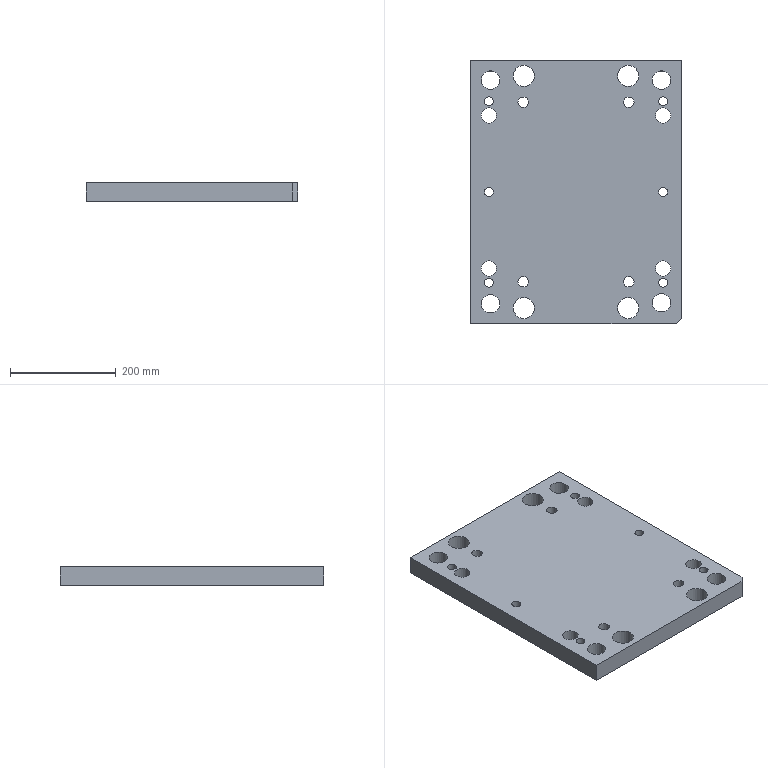Part | STEP file | SL2-MOLD_id734_xmt_txt | 1 solid | 29 faces | box 400 x 500 x 35 mm | volume 6503504 mm3 | cylinder 22 | plane 7 | commonest cylinder face diameters 17 x6 20 x4 29 x4 35 x4 40 x4
STEP:
#1=CARTESIAN_POINT('',(-200.,-160.,-114.));
#2=VERTEX_POINT('',#1);
#3=CARTESIAN_POINT('',(190.,-160.,-114.));
#4=VERTEX_POINT('',#3);
#5=CARTESIAN_POINT('',(0.,-160.,-114.));
#6=DIRECTION('',(1.,0.,0.));
#7=VECTOR('',#6,1.);
#8=LINE('',#5,#7);
#9=EDGE_CURVE('',#2,#4,#8,.T.);
#10=ORIENTED_EDGE('',*,*,#9,.T.);
#11=CARTESIAN_POINT('',(190.,-160.,-79.));
#12=VERTEX_POINT('',#11);
#13=CARTESIAN_POINT('',(190.,-160.,-114.));
#14=DIRECTION('',(0.,0.,1.));
#15=VECTOR('',#14,1.);
#16=LINE('',#13,#15);
#17=EDGE_CURVE('',#4,#12,#16,.T.);
#18=ORIENTED_EDGE('',*,*,#17,.T.);
#19=CARTESIAN_POINT('',(-200.,-160.,-79.));
#20=VERTEX_POINT('',#19);
#21=CARTESIAN_POINT('',(0.,-160.,-79.));
#22=DIRECTION('',(1.,0.,0.));
#23=VECTOR('',#22,1.);
#24=LINE('',#21,#23);
#25=EDGE_CURVE('',#20,#12,#24,.T.);
#26=ORIENTED_EDGE('',*,*,#25,.F.);
#27=CARTESIAN_POINT('',(-200.,-160.,-114.));
#28=DIRECTION('',(0.,0.,1.));
#29=VECTOR('',#28,1.);
#30=LINE('',#27,#29);
#31=EDGE_CURVE('',#2,#20,#30,.T.);
#32=ORIENTED_EDGE('',*,*,#31,.F.);
#33=EDGE_LOOP('',(#10,#18,#26,#32));
#34=FACE_OUTER_BOUND('',#33,.T.);
#35=CARTESIAN_POINT('',(0.,-160.,-114.));
#36=DIRECTION('',(0.,-1.,0.));
#37=DIRECTION('',(0.,0.,-1.));
#38=AXIS2_PLACEMENT_3D('',#35,#36,#37);
#39=PLANE('',#38);
#40=ADVANCED_FACE('',(#34),#39,.T.);
#41=CARTESIAN_POINT('',(-200.,340.,-79.));
#42=VERTEX_POINT('',#41);
#43=CARTESIAN_POINT('',(-200.,0.,-79.));
#44=DIRECTION('',(0.,-1.,0.));
#45=VECTOR('',#44,1.);
#46=LINE('',#43,#45);
#47=EDGE_CURVE('',#42,#20,#46,.T.);
#48=ORIENTED_EDGE('',*,*,#47,.F.);
#49=CARTESIAN_POINT('',(-200.,340.,-114.));
#50=VERTEX_POINT('',#49);
#51=CARTESIAN_POINT('',(-200.,340.,-114.));
#52=DIRECTION('',(0.,0.,1.));
#53=VECTOR('',#52,1.);
#54=LINE('',#51,#53);
#55=EDGE_CURVE('',#50,#42,#54,.T.);
#56=ORIENTED_EDGE('',*,*,#55,.F.);
#57=CARTESIAN_POINT('',(-200.,0.,-114.));
#58=DIRECTION('',(0.,-1.,0.));
#59=VECTOR('',#58,1.);
#60=LINE('',#57,#59);
#61=EDGE_CURVE('',#50,#2,#60,.T.);
#62=ORIENTED_EDGE('',*,*,#61,.T.);
#63=ORIENTED_EDGE('',*,*,#31,.T.);
#64=EDGE_LOOP('',(#48,#56,#62,#63));
#65=FACE_OUTER_BOUND('',#64,.T.);
#66=CARTESIAN_POINT('',(-200.,0.,-114.));
#67=DIRECTION('',(-1.,0.,0.));
#68=DIRECTION('',(0.,0.,1.));
#69=AXIS2_PLACEMENT_3D('',#66,#67,#68);
#70=PLANE('',#69);
#71=ADVANCED_FACE('',(#65),#70,.T.);
#72=CARTESIAN_POINT('',(200.,340.,-79.));
#73=VERTEX_POINT('',#72);
#74=CARTESIAN_POINT('',(0.,340.,-79.));
#75=DIRECTION('',(-1.,0.,0.));
#76=VECTOR('',#75,1.);
#77=LINE('',#74,#76);
#78=EDGE_CURVE('',#73,#42,#77,.T.);
#79=ORIENTED_EDGE('',*,*,#78,.F.);
#80=CARTESIAN_POINT('',(200.,340.,-114.));
#81=VERTEX_POINT('',#80);
#82=CARTESIAN_POINT('',(200.,340.,-114.));
#83=DIRECTION('',(0.,0.,1.));
#84=VECTOR('',#83,1.);
#85=LINE('',#82,#84);
#86=EDGE_CURVE('',#81,#73,#85,.T.);
#87=ORIENTED_EDGE('',*,*,#86,.F.);
#88=CARTESIAN_POINT('',(0.,340.,-114.));
#89=DIRECTION('',(-1.,0.,0.));
#90=VECTOR('',#89,1.);
#91=LINE('',#88,#90);
#92=EDGE_CURVE('',#81,#50,#91,.T.);
#93=ORIENTED_EDGE('',*,*,#92,.T.);
#94=ORIENTED_EDGE('',*,*,#55,.T.);
#95=EDGE_LOOP('',(#79,#87,#93,#94));
#96=FACE_OUTER_BOUND('',#95,.T.);
#97=CARTESIAN_POINT('',(0.,340.,-114.));
#98=DIRECTION('',(0.,1.,0.));
#99=DIRECTION('',(0.,0.,1.));
#100=AXIS2_PLACEMENT_3D('',#97,#98,#99);
#101=PLANE('',#100);
#102=ADVANCED_FACE('',(#96),#101,.T.);
#103=CARTESIAN_POINT('',(200.,-150.,-79.));
#104=VERTEX_POINT('',#103);
#105=CARTESIAN_POINT('',(200.,0.,-79.));
#106=DIRECTION('',(0.,1.,0.));
#107=VECTOR('',#106,1.);
#108=LINE('',#105,#107);
#109=EDGE_CURVE('',#104,#73,#108,.T.);
#110=ORIENTED_EDGE('',*,*,#109,.F.);
#111=CARTESIAN_POINT('',(200.,-150.,-114.));
#112=VERTEX_POINT('',#111);
#113=CARTESIAN_POINT('',(200.,-150.,-114.));
#114=DIRECTION('',(0.,0.,-1.));
#115=VECTOR('',#114,1.);
#116=LINE('',#113,#115);
#117=EDGE_CURVE('',#104,#112,#116,.T.);
#118=ORIENTED_EDGE('',*,*,#117,.T.);
#119=CARTESIAN_POINT('',(200.,0.,-114.));
#120=DIRECTION('',(0.,1.,0.));
#121=VECTOR('',#120,1.);
#122=LINE('',#119,#121);
#123=EDGE_CURVE('',#112,#81,#122,.T.);
#124=ORIENTED_EDGE('',*,*,#123,.T.);
#125=ORIENTED_EDGE('',*,*,#86,.T.);
#126=EDGE_LOOP('',(#110,#118,#124,#125));
#127=FACE_OUTER_BOUND('',#126,.T.);
#128=CARTESIAN_POINT('',(200.,0.,-114.));
#129=DIRECTION('',(1.,0.,0.));
#130=DIRECTION('',(0.,0.,-1.));
#131=AXIS2_PLACEMENT_3D('',#128,#129,#130);
#132=PLANE('',#131);
#133=ADVANCED_FACE('',(#127),#132,.T.);
#134=CARTESIAN_POINT('',(-90.,260.,-114.));
#135=VERTEX_POINT('',#134);
#136=CARTESIAN_POINT('',(-100.,260.,-114.));
#137=DIRECTION('',(0.,0.,-1.));
#138=DIRECTION('',(1.,0.,0.));
#139=AXIS2_PLACEMENT_3D('',#136,#137,#138);
#140=CIRCLE('',#139,10.);
#141=EDGE_CURVE('',#135,#135,#140,.T.);
#142=ORIENTED_EDGE('',*,*,#141,.F.);
#143=EDGE_LOOP('',(#142));
#144=FACE_BOUND('',#143,.T.);
#145=CARTESIAN_POINT('',(110.,-80.,-114.));
#146=VERTEX_POINT('',#145);
#147=CARTESIAN_POINT('',(100.,-80.,-114.));
#148=DIRECTION('',(0.,0.,-1.));
#149=DIRECTION('',(1.,0.,0.));
#150=AXIS2_PLACEMENT_3D('',#147,#148,#149);
#151=CIRCLE('',#150,10.);
#152=EDGE_CURVE('',#146,#146,#151,.T.);
#153=ORIENTED_EDGE('',*,*,#152,.F.);
#154=EDGE_LOOP('',(#153));
#155=FACE_BOUND('',#154,.T.);
#156=CARTESIAN_POINT('',(-90.,-80.,-114.));
#157=VERTEX_POINT('',#156);
#158=CARTESIAN_POINT('',(-100.,-80.,-114.));
#159=DIRECTION('',(0.,0.,-1.));
#160=DIRECTION('',(1.,0.,0.));
#161=AXIS2_PLACEMENT_3D('',#158,#159,#160);
#162=CIRCLE('',#161,10.);
#163=EDGE_CURVE('',#157,#157,#162,.T.);
#164=ORIENTED_EDGE('',*,*,#163,.F.);
#165=EDGE_LOOP('',(#164));
#166=FACE_BOUND('',#165,.T.);
#167=CARTESIAN_POINT('',(110.,260.,-114.));
#168=VERTEX_POINT('',#167);
#169=CARTESIAN_POINT('',(100.,260.,-114.));
#170=DIRECTION('',(0.,0.,-1.));
#171=DIRECTION('',(1.,0.,0.));
#172=AXIS2_PLACEMENT_3D('',#169,#170,#171);
#173=CIRCLE('',#172,10.);
#174=EDGE_CURVE('',#168,#168,#173,.T.);
#175=ORIENTED_EDGE('',*,*,#174,.F.);
#176=EDGE_LOOP('',(#175));
#177=FACE_BOUND('',#176,.T.);
#178=CARTESIAN_POINT('',(-79.,310.,-114.));
#179=VERTEX_POINT('',#178);
#180=CARTESIAN_POINT('',(-99.,310.,-114.));
#181=DIRECTION('',(0.,0.,-1.));
#182=DIRECTION('',(1.,0.,0.));
#183=AXIS2_PLACEMENT_3D('',#180,#181,#182);
#184=CIRCLE('',#183,20.);
#185=EDGE_CURVE('',#179,#179,#184,.T.);
#186=ORIENTED_EDGE('',*,*,#185,.F.);
#187=EDGE_LOOP('',(#186));
#188=FACE_BOUND('',#187,.T.);
#189=CARTESIAN_POINT('',(119.,310.,-114.));
#190=VERTEX_POINT('',#189);
#191=CARTESIAN_POINT('',(99.,310.,-114.));
#192=DIRECTION('',(0.,0.,-1.));
#193=DIRECTION('',(1.,0.,0.));
#194=AXIS2_PLACEMENT_3D('',#191,#192,#193);
#195=CIRCLE('',#194,20.);
#196=EDGE_CURVE('',#190,#190,#195,.T.);
#197=ORIENTED_EDGE('',*,*,#196,.F.);
#198=EDGE_LOOP('',(#197));
#199=FACE_BOUND('',#198,.T.);
#200=CARTESIAN_POINT('',(119.,-130.,-114.));
#201=VERTEX_POINT('',#200);
#202=CARTESIAN_POINT('',(99.,-130.,-114.));
#203=DIRECTION('',(0.,0.,-1.));
#204=DIRECTION('',(1.,0.,0.));
#205=AXIS2_PLACEMENT_3D('',#202,#203,#204);
#206=CIRCLE('',#205,20.);
#207=EDGE_CURVE('',#201,#201,#206,.T.);
#208=ORIENTED_EDGE('',*,*,#207,.F.);
#209=EDGE_LOOP('',(#208));
#210=FACE_BOUND('',#209,.T.);
#211=CARTESIAN_POINT('',(-79.,-130.,-114.));
#212=VERTEX_POINT('',#211);
#213=CARTESIAN_POINT('',(-99.,-130.,-114.));
#214=DIRECTION('',(0.,0.,-1.));
#215=DIRECTION('',(1.,0.,0.));
#216=AXIS2_PLACEMENT_3D('',#213,#214,#215);
#217=CIRCLE('',#216,20.);
#218=EDGE_CURVE('',#212,#212,#217,.T.);
#219=ORIENTED_EDGE('',*,*,#218,.F.);
#220=EDGE_LOOP('',(#219));
#221=FACE_BOUND('',#220,.T.);
#222=CARTESIAN_POINT('',(-156.5,-82.,-114.));
#223=VERTEX_POINT('',#222);
#224=CARTESIAN_POINT('',(-165.,-82.,-114.));
#225=DIRECTION('',(0.,0.,1.));
#226=DIRECTION('',(1.,0.,0.));
#227=AXIS2_PLACEMENT_3D('',#224,#225,#226);
#228=CIRCLE('',#227,8.5);
#229=EDGE_CURVE('',#223,#223,#228,.T.);
#230=ORIENTED_EDGE('',*,*,#229,.T.);
#231=EDGE_LOOP('',(#230));
#232=FACE_BOUND('',#231,.T.);
#233=CARTESIAN_POINT('',(-156.5,90.,-114.));
#234=VERTEX_POINT('',#233);
#235=CARTESIAN_POINT('',(-165.,90.,-114.));
#236=DIRECTION('',(0.,0.,1.));
#237=DIRECTION('',(1.,0.,0.));
#238=AXIS2_PLACEMENT_3D('',#235,#236,#237);
#239=CIRCLE('',#238,8.5);
#240=EDGE_CURVE('',#234,#234,#239,.T.);
#241=ORIENTED_EDGE('',*,*,#240,.T.);
#242=EDGE_LOOP('',(#241));
#243=FACE_BOUND('',#242,.T.);
#244=CARTESIAN_POINT('',(-156.5,262.,-114.));
#245=VERTEX_POINT('',#244);
#246=CARTESIAN_POINT('',(-165.,262.,-114.));
#247=DIRECTION('',(0.,0.,1.));
#248=DIRECTION('',(1.,0.,0.));
#249=AXIS2_PLACEMENT_3D('',#246,#247,#248);
#250=CIRCLE('',#249,8.5);
#251=EDGE_CURVE('',#245,#245,#250,.T.);
#252=ORIENTED_EDGE('',*,*,#251,.T.);
#253=EDGE_LOOP('',(#252));
#254=FACE_BOUND('',#253,.T.);
#255=CARTESIAN_POINT('',(173.5,262.,-114.));
#256=VERTEX_POINT('',#255);
#257=CARTESIAN_POINT('',(165.,262.,-114.));
#258=DIRECTION('',(0.,0.,1.));
#259=DIRECTION('',(1.,0.,0.));
#260=AXIS2_PLACEMENT_3D('',#257,#258,#259);
#261=CIRCLE('',#260,8.5);
#262=EDGE_CURVE('',#256,#256,#261,.T.);
#263=ORIENTED_EDGE('',*,*,#262,.T.);
#264=EDGE_LOOP('',(#263));
#265=FACE_BOUND('',#264,.T.);
#266=CARTESIAN_POINT('',(173.5,90.,-114.));
#267=VERTEX_POINT('',#266);
#268=CARTESIAN_POINT('',(165.,90.,-114.));
#269=DIRECTION('',(0.,0.,1.));
#270=DIRECTION('',(1.,0.,0.));
#271=AXIS2_PLACEMENT_3D('',#268,#269,#270);
#272=CIRCLE('',#271,8.5);
#273=EDGE_CURVE('',#267,#267,#272,.T.);
#274=ORIENTED_EDGE('',*,*,#273,.T.);
#275=EDGE_LOOP('',(#274));
#276=FACE_BOUND('',#275,.T.);
#277=CARTESIAN_POINT('',(173.5,-82.,-114.));
#278=VERTEX_POINT('',#277);
#279=CARTESIAN_POINT('',(165.,-82.,-114.));
#280=DIRECTION('',(0.,0.,1.));
#281=DIRECTION('',(1.,0.,0.));
#282=AXIS2_PLACEMENT_3D('',#279,#280,#281);
#283=CIRCLE('',#282,8.5);
#284=EDGE_CURVE('',#278,#278,#283,.T.);
#285=ORIENTED_EDGE('',*,*,#284,.T.);
#286=EDGE_LOOP('',(#285));
#287=FACE_BOUND('',#286,.T.);
#288=CARTESIAN_POINT('',(-150.5,-55.,-114.));
#289=VERTEX_POINT('',#288);
#290=CARTESIAN_POINT('',(-165.,-55.,-114.));
#291=DIRECTION('',(0.,0.,1.));
#292=DIRECTION('',(1.,0.,0.));
#293=AXIS2_PLACEMENT_3D('',#290,#291,#292);
#294=CIRCLE('',#293,14.5);
#295=EDGE_CURVE('',#289,#289,#294,.T.);
#296=ORIENTED_EDGE('',*,*,#295,.T.);
#297=EDGE_LOOP('',(#296));
#298=FACE_BOUND('',#297,.T.);
#299=CARTESIAN_POINT('',(179.5,-55.,-114.));
#300=VERTEX_POINT('',#299);
#301=CARTESIAN_POINT('',(165.,-55.,-114.));
#302=DIRECTION('',(0.,0.,1.));
#303=DIRECTION('',(1.,0.,0.));
#304=AXIS2_PLACEMENT_3D('',#301,#302,#303);
#305=CIRCLE('',#304,14.5);
#306=EDGE_CURVE('',#300,#300,#305,.T.);
#307=ORIENTED_EDGE('',*,*,#306,.T.);
#308=EDGE_LOOP('',(#307));
#309=FACE_BOUND('',#308,.T.);
#310=CARTESIAN_POINT('',(179.5,235.,-114.));
#311=VERTEX_POINT('',#310);
#312=CARTESIAN_POINT('',(165.,235.,-114.));
#313=DIRECTION('',(0.,0.,1.));
#314=DIRECTION('',(1.,0.,0.));
#315=AXIS2_PLACEMENT_3D('',#312,#313,#314);
#316=CIRCLE('',#315,14.5);
#317=EDGE_CURVE('',#311,#311,#316,.T.);
#318=ORIENTED_EDGE('',*,*,#317,.T.);
#319=EDGE_LOOP('',(#318));
#320=FACE_BOUND('',#319,.T.);
#321=CARTESIAN_POINT('',(-150.5,235.,-114.));
#322=VERTEX_POINT('',#321);
#323=CARTESIAN_POINT('',(-165.,235.,-114.));
#324=DIRECTION('',(0.,0.,1.));
#325=DIRECTION('',(1.,0.,0.));
#326=AXIS2_PLACEMENT_3D('',#323,#324,#325);
#327=CIRCLE('',#326,14.5);
#328=EDGE_CURVE('',#322,#322,#327,.T.);
#329=ORIENTED_EDGE('',*,*,#328,.T.);
#330=EDGE_LOOP('',(#329));
#331=FACE_BOUND('',#330,.T.);
#332=CARTESIAN_POINT('',(-144.5,-122.,-114.));
#333=VERTEX_POINT('',#332);
#334=CARTESIAN_POINT('',(-162.,-122.,-114.));
#335=DIRECTION('',(0.,0.,-1.));
#336=DIRECTION('',(1.,0.,0.));
#337=AXIS2_PLACEMENT_3D('',#334,#335,#336);
#338=CIRCLE('',#337,17.5);
#339=EDGE_CURVE('',#333,#333,#338,.T.);
#340=ORIENTED_EDGE('',*,*,#339,.F.);
#341=EDGE_LOOP('',(#340));
#342=FACE_BOUND('',#341,.T.);
#343=CARTESIAN_POINT('',(179.5,-120.,-114.));
#344=VERTEX_POINT('',#343);
#345=CARTESIAN_POINT('',(162.,-120.,-114.));
#346=DIRECTION('',(0.,0.,-1.));
#347=DIRECTION('',(1.,0.,0.));
#348=AXIS2_PLACEMENT_3D('',#345,#346,#347);
#349=CIRCLE('',#348,17.5);
#350=EDGE_CURVE('',#344,#344,#349,.T.);
#351=ORIENTED_EDGE('',*,*,#350,.F.);
#352=EDGE_LOOP('',(#351));
#353=FACE_BOUND('',#352,.T.);
#354=CARTESIAN_POINT('',(179.5,302.,-114.));
#355=VERTEX_POINT('',#354);
#356=CARTESIAN_POINT('',(162.,302.,-114.));
#357=DIRECTION('',(0.,0.,-1.));
#358=DIRECTION('',(1.,0.,0.));
#359=AXIS2_PLACEMENT_3D('',#356,#357,#358);
#360=CIRCLE('',#359,17.5);
#361=EDGE_CURVE('',#355,#355,#360,.T.);
#362=ORIENTED_EDGE('',*,*,#361,.F.);
#363=EDGE_LOOP('',(#362));
#364=FACE_BOUND('',#363,.T.);
#365=CARTESIAN_POINT('',(-144.5,302.,-114.));
#366=VERTEX_POINT('',#365);
#367=CARTESIAN_POINT('',(-162.,302.,-114.));
#368=DIRECTION('',(0.,0.,-1.));
#369=DIRECTION('',(1.,0.,0.));
#370=AXIS2_PLACEMENT_3D('',#367,#368,#369);
#371=CIRCLE('',#370,17.5);
#372=EDGE_CURVE('',#366,#366,#371,.T.);
#373=ORIENTED_EDGE('',*,*,#372,.F.);
#374=EDGE_LOOP('',(#373));
#375=FACE_BOUND('',#374,.T.);
#376=ORIENTED_EDGE('',*,*,#123,.F.);
#377=CARTESIAN_POINT('',(190.,-160.,-114.));
#378=DIRECTION('',(-0.7071,-0.7071,0.));
#379=VECTOR('',#378,1.);
#380=LINE('',#377,#379);
#381=EDGE_CURVE('',#112,#4,#380,.T.);
#382=ORIENTED_EDGE('',*,*,#381,.T.);
#383=ORIENTED_EDGE('',*,*,#9,.F.);
#384=ORIENTED_EDGE('',*,*,#61,.F.);
#385=ORIENTED_EDGE('',*,*,#92,.F.);
#386=EDGE_LOOP('',(#376,#382,#383,#384,#385));
#387=FACE_BOUND('',#386,.T.);
#388=CARTESIAN_POINT('',(0.,0.,-114.));
#389=DIRECTION('',(0.,0.,1.));
#390=DIRECTION('',(1.,0.,0.));
#391=AXIS2_PLACEMENT_3D('',#388,#389,#390);
#392=PLANE('',#391);
#393=ADVANCED_FACE('',(#144,#155,#166,#177,#188,#199,#210,#221,#232,#243,#254,#265,#276,#287,#298,#309,#320,#331,#342,#353,#364,#375,#387),#392,.F.);
#394=CARTESIAN_POINT('',(-90.,260.,-79.));
#395=VERTEX_POINT('',#394);
#396=CARTESIAN_POINT('',(-100.,260.,-79.));
#397=DIRECTION('',(0.,0.,-1.));
#398=DIRECTION('',(1.,0.,0.));
#399=AXIS2_PLACEMENT_3D('',#396,#397,#398);
#400=CIRCLE('',#399,10.);
#401=EDGE_CURVE('',#395,#395,#400,.T.);
#402=ORIENTED_EDGE('',*,*,#401,.T.);
#403=EDGE_LOOP('',(#402));
#404=FACE_BOUND('',#403,.T.);
#405=CARTESIAN_POINT('',(110.,-80.,-79.));
#406=VERTEX_POINT('',#405);
#407=CARTESIAN_POINT('',(100.,-80.,-79.));
#408=DIRECTION('',(0.,0.,-1.));
#409=DIRECTION('',(1.,0.,0.));
#410=AXIS2_PLACEMENT_3D('',#407,#408,#409);
#411=CIRCLE('',#410,10.);
#412=EDGE_CURVE('',#406,#406,#411,.T.);
#413=ORIENTED_EDGE('',*,*,#412,.T.);
#414=EDGE_LOOP('',(#413));
#415=FACE_BOUND('',#414,.T.);
#416=CARTESIAN_POINT('',(-90.,-80.,-79.));
#417=VERTEX_POINT('',#416);
#418=CARTESIAN_POINT('',(-100.,-80.,-79.));
#419=DIRECTION('',(0.,0.,-1.));
#420=DIRECTION('',(1.,0.,0.));
#421=AXIS2_PLACEMENT_3D('',#418,#419,#420);
#422=CIRCLE('',#421,10.);
#423=EDGE_CURVE('',#417,#417,#422,.T.);
#424=ORIENTED_EDGE('',*,*,#423,.T.);
#425=EDGE_LOOP('',(#424));
#426=FACE_BOUND('',#425,.T.);
#427=CARTESIAN_POINT('',(110.,260.,-79.));
#428=VERTEX_POINT('',#427);
#429=CARTESIAN_POINT('',(100.,260.,-79.));
#430=DIRECTION('',(0.,0.,-1.));
#431=DIRECTION('',(1.,0.,0.));
#432=AXIS2_PLACEMENT_3D('',#429,#430,#431);
#433=CIRCLE('',#432,10.);
#434=EDGE_CURVE('',#428,#428,#433,.T.);
#435=ORIENTED_EDGE('',*,*,#434,.T.);
#436=EDGE_LOOP('',(#435));
#437=FACE_BOUND('',#436,.T.);
#438=CARTESIAN_POINT('',(-79.,310.,-79.));
#439=VERTEX_POINT('',#438);
#440=CARTESIAN_POINT('',(-99.,310.,-79.));
#441=DIRECTION('',(0.,0.,-1.));
#442=DIRECTION('',(1.,0.,0.));
#443=AXIS2_PLACEMENT_3D('',#440,#441,#442);
#444=CIRCLE('',#443,20.);
#445=EDGE_CURVE('',#439,#439,#444,.T.);
#446=ORIENTED_EDGE('',*,*,#445,.T.);
#447=EDGE_LOOP('',(#446));
#448=FACE_BOUND('',#447,.T.);
#449=CARTESIAN_POINT('',(119.,310.,-79.));
#450=VERTEX_POINT('',#449);
#451=CARTESIAN_POINT('',(99.,310.,-79.));
#452=DIRECTION('',(0.,0.,-1.));
#453=DIRECTION('',(1.,0.,0.));
#454=AXIS2_PLACEMENT_3D('',#451,#452,#453);
#455=CIRCLE('',#454,20.);
#456=EDGE_CURVE('',#450,#450,#455,.T.);
#457=ORIENTED_EDGE('',*,*,#456,.T.);
#458=EDGE_LOOP('',(#457));
#459=FACE_BOUND('',#458,.T.);
#460=CARTESIAN_POINT('',(119.,-130.,-79.));
#461=VERTEX_POINT('',#460);
#462=CARTESIAN_POINT('',(99.,-130.,-79.));
#463=DIRECTION('',(0.,0.,-1.));
#464=DIRECTION('',(1.,0.,0.));
#465=AXIS2_PLACEMENT_3D('',#462,#463,#464);
#466=CIRCLE('',#465,20.);
#467=EDGE_CURVE('',#461,#461,#466,.T.);
#468=ORIENTED_EDGE('',*,*,#467,.T.);
#469=EDGE_LOOP('',(#468));
#470=FACE_BOUND('',#469,.T.);
#471=CARTESIAN_POINT('',(-79.,-130.,-79.));
#472=VERTEX_POINT('',#471);
#473=CARTESIAN_POINT('',(-99.,-130.,-79.));
#474=DIRECTION('',(0.,0.,-1.));
#475=DIRECTION('',(1.,0.,0.));
#476=AXIS2_PLACEMENT_3D('',#473,#474,#475);
#477=CIRCLE('',#476,20.);
#478=EDGE_CURVE('',#472,#472,#477,.T.);
#479=ORIENTED_EDGE('',*,*,#478,.T.);
#480=EDGE_LOOP('',(#479));
#481=FACE_BOUND('',#480,.T.);
#482=CARTESIAN_POINT('',(-156.5,-82.,-79.));
#483=VERTEX_POINT('',#482);
#484=CARTESIAN_POINT('',(-165.,-82.,-79.));
#485=DIRECTION('',(0.,0.,1.));
#486=DIRECTION('',(1.,0.,0.));
#487=AXIS2_PLACEMENT_3D('',#484,#485,#486);
#488=CIRCLE('',#487,8.5);
#489=EDGE_CURVE('',#483,#483,#488,.T.);
#490=ORIENTED_EDGE('',*,*,#489,.F.);
#491=EDGE_LOOP('',(#490));
#492=FACE_BOUND('',#491,.T.);
#493=CARTESIAN_POINT('',(-156.5,90.,-79.));
#494=VERTEX_POINT('',#493);
#495=CARTESIAN_POINT('',(-165.,90.,-79.));
#496=DIRECTION('',(0.,0.,1.));
#497=DIRECTION('',(1.,0.,0.));
#498=AXIS2_PLACEMENT_3D('',#495,#496,#497);
#499=CIRCLE('',#498,8.5);
#500=EDGE_CURVE('',#494,#494,#499,.T.);
#501=ORIENTED_EDGE('',*,*,#500,.F.);
#502=EDGE_LOOP('',(#501));
#503=FACE_BOUND('',#502,.T.);
#504=CARTESIAN_POINT('',(-156.5,262.,-79.));
#505=VERTEX_POINT('',#504);
#506=CARTESIAN_POINT('',(-165.,262.,-79.));
#507=DIRECTION('',(0.,0.,1.));
#508=DIRECTION('',(1.,0.,0.));
#509=AXIS2_PLACEMENT_3D('',#506,#507,#508);
#510=CIRCLE('',#509,8.5);
#511=EDGE_CURVE('',#505,#505,#510,.T.);
#512=ORIENTED_EDGE('',*,*,#511,.F.);
#513=EDGE_LOOP('',(#512));
#514=FACE_BOUND('',#513,.T.);
#515=CARTESIAN_POINT('',(173.5,262.,-79.));
#516=VERTEX_POINT('',#515);
#517=CARTESIAN_POINT('',(165.,262.,-79.));
#518=DIRECTION('',(0.,0.,1.));
#519=DIRECTION('',(1.,0.,0.));
#520=AXIS2_PLACEMENT_3D('',#517,#518,#519);
#521=CIRCLE('',#520,8.5);
#522=EDGE_CURVE('',#516,#516,#521,.T.);
#523=ORIENTED_EDGE('',*,*,#522,.F.);
#524=EDGE_LOOP('',(#523));
#525=FACE_BOUND('',#524,.T.);
#526=CARTESIAN_POINT('',(173.5,90.,-79.));
#527=VERTEX_POINT('',#526);
#528=CARTESIAN_POINT('',(165.,90.,-79.));
#529=DIRECTION('',(0.,0.,1.));
#530=DIRECTION('',(1.,0.,0.));
#531=AXIS2_PLACEMENT_3D('',#528,#529,#530);
#532=CIRCLE('',#531,8.5);
#533=EDGE_CURVE('',#527,#527,#532,.T.);
#534=ORIENTED_EDGE('',*,*,#533,.F.);
#535=EDGE_LOOP('',(#534));
#536=FACE_BOUND('',#535,.T.);
#537=CARTESIAN_POINT('',(173.5,-82.,-79.));
#538=VERTEX_POINT('',#537);
#539=CARTESIAN_POINT('',(165.,-82.,-79.));
#540=DIRECTION('',(0.,0.,1.));
#541=DIRECTION('',(1.,0.,0.));
#542=AXIS2_PLACEMENT_3D('',#539,#540,#541);
#543=CIRCLE('',#542,8.5);
#544=EDGE_CURVE('',#538,#538,#543,.T.);
#545=ORIENTED_EDGE('',*,*,#544,.F.);
#546=EDGE_LOOP('',(#545));
#547=FACE_BOUND('',#546,.T.);
#548=CARTESIAN_POINT('',(-150.5,-55.,-79.));
#549=VERTEX_POINT('',#548);
#550=CARTESIAN_POINT('',(-165.,-55.,-79.));
#551=DIRECTION('',(0.,0.,1.));
#552=DIRECTION('',(1.,0.,0.));
#553=AXIS2_PLACEMENT_3D('',#550,#551,#552);
#554=CIRCLE('',#553,14.5);
#555=EDGE_CURVE('',#549,#549,#554,.T.);
#556=ORIENTED_EDGE('',*,*,#555,.F.);
#557=EDGE_LOOP('',(#556));
#558=FACE_BOUND('',#557,.T.);
#559=CARTESIAN_POINT('',(179.5,-55.,-79.));
#560=VERTEX_POINT('',#559);
#561=CARTESIAN_POINT('',(165.,-55.,-79.));
#562=DIRECTION('',(0.,0.,1.));
#563=DIRECTION('',(1.,0.,0.));
#564=AXIS2_PLACEMENT_3D('',#561,#562,#563);
#565=CIRCLE('',#564,14.5);
#566=EDGE_CURVE('',#560,#560,#565,.T.);
#567=ORIENTED_EDGE('',*,*,#566,.F.);
#568=EDGE_LOOP('',(#567));
#569=FACE_BOUND('',#568,.T.);
#570=CARTESIAN_POINT('',(179.5,235.,-79.));
#571=VERTEX_POINT('',#570);
#572=CARTESIAN_POINT('',(165.,235.,-79.));
#573=DIRECTION('',(0.,0.,1.));
#574=DIRECTION('',(1.,0.,0.));
#575=AXIS2_PLACEMENT_3D('',#572,#573,#574);
#576=CIRCLE('',#575,14.5);
#577=EDGE_CURVE('',#571,#571,#576,.T.);
#578=ORIENTED_EDGE('',*,*,#577,.F.);
#579=EDGE_LOOP('',(#578));
#580=FACE_BOUND('',#579,.T.);
#581=CARTESIAN_POINT('',(-150.5,235.,-79.));
#582=VERTEX_POINT('',#581);
#583=CARTESIAN_POINT('',(-165.,235.,-79.));
#584=DIRECTION('',(0.,0.,1.));
#585=DIRECTION('',(1.,0.,0.));
#586=AXIS2_PLACEMENT_3D('',#583,#584,#585);
#587=CIRCLE('',#586,14.5);
#588=EDGE_CURVE('',#582,#582,#587,.T.);
#589=ORIENTED_EDGE('',*,*,#588,.F.);
#590=EDGE_LOOP('',(#589));
#591=FACE_BOUND('',#590,.T.);
#592=CARTESIAN_POINT('',(-144.5,-122.,-79.));
#593=VERTEX_POINT('',#592);
#594=CARTESIAN_POINT('',(-162.,-122.,-79.));
#595=DIRECTION('',(0.,0.,-1.));
#596=DIRECTION('',(1.,0.,0.));
#597=AXIS2_PLACEMENT_3D('',#594,#595,#596);
#598=CIRCLE('',#597,17.5);
#599=EDGE_CURVE('',#593,#593,#598,.T.);
#600=ORIENTED_EDGE('',*,*,#599,.T.);
#601=EDGE_LOOP('',(#600));
#602=FACE_BOUND('',#601,.T.);
#603=CARTESIAN_POINT('',(179.5,-120.,-79.));
#604=VERTEX_POINT('',#603);
#605=CARTESIAN_POINT('',(162.,-120.,-79.));
#606=DIRECTION('',(0.,0.,-1.));
#607=DIRECTION('',(1.,0.,0.));
#608=AXIS2_PLACEMENT_3D('',#605,#606,#607);
#609=CIRCLE('',#608,17.5);
#610=EDGE_CURVE('',#604,#604,#609,.T.);
#611=ORIENTED_EDGE('',*,*,#610,.T.);
#612=EDGE_LOOP('',(#611));
#613=FACE_BOUND('',#612,.T.);
#614=CARTESIAN_POINT('',(179.5,302.,-79.));
#615=VERTEX_POINT('',#614);
#616=CARTESIAN_POINT('',(162.,302.,-79.));
#617=DIRECTION('',(0.,0.,-1.));
#618=DIRECTION('',(1.,0.,0.));
#619=AXIS2_PLACEMENT_3D('',#616,#617,#618);
#620=CIRCLE('',#619,17.5);
#621=EDGE_CURVE('',#615,#615,#620,.T.);
#622=ORIENTED_EDGE('',*,*,#621,.T.);
#623=EDGE_LOOP('',(#622));
#624=FACE_BOUND('',#623,.T.);
#625=CARTESIAN_POINT('',(-144.5,302.,-79.));
#626=VERTEX_POINT('',#625);
#627=CARTESIAN_POINT('',(-162.,302.,-79.));
#628=DIRECTION('',(0.,0.,-1.));
#629=DIRECTION('',(1.,0.,0.));
#630=AXIS2_PLACEMENT_3D('',#627,#628,#629);
#631=CIRCLE('',#630,17.5);
#632=EDGE_CURVE('',#626,#626,#631,.T.);
#633=ORIENTED_EDGE('',*,*,#632,.T.);
#634=EDGE_LOOP('',(#633));
#635=FACE_BOUND('',#634,.T.);
#636=ORIENTED_EDGE('',*,*,#25,.T.);
#637=CARTESIAN_POINT('',(175.,-175.,-79.));
#638=DIRECTION('',(0.7071,0.7071,0.));
#639=VECTOR('',#638,1.);
#640=LINE('',#637,#639);
#641=EDGE_CURVE('',#12,#104,#640,.T.);
#642=ORIENTED_EDGE('',*,*,#641,.T.);
#643=ORIENTED_EDGE('',*,*,#109,.T.);
#644=ORIENTED_EDGE('',*,*,#78,.T.);
#645=ORIENTED_EDGE('',*,*,#47,.T.);
#646=EDGE_LOOP('',(#636,#642,#643,#644,#645));
#647=FACE_BOUND('',#646,.T.);
#648=CARTESIAN_POINT('',(0.,0.,-79.));
#649=DIRECTION('',(0.,0.,1.));
#650=DIRECTION('',(1.,0.,0.));
#651=AXIS2_PLACEMENT_3D('',#648,#649,#650);
#652=PLANE('',#651);
#653=ADVANCED_FACE('',(#404,#415,#426,#437,#448,#459,#470,#481,#492,#503,#514,#525,#536,#547,#558,#569,#580,#591,#602,#613,#624,#635,#647),#652,.T.);
#654=ORIENTED_EDGE('',*,*,#381,.F.);
#655=ORIENTED_EDGE('',*,*,#117,.F.);
#656=ORIENTED_EDGE('',*,*,#641,.F.);
#657=ORIENTED_EDGE('',*,*,#17,.F.);
#658=EDGE_LOOP('',(#654,#655,#656,#657));
#659=FACE_OUTER_BOUND('',#658,.T.);
#660=CARTESIAN_POINT('',(190.,-160.,-114.));
#661=DIRECTION('',(-0.7071,0.7071,0.));
#662=DIRECTION('',(0.,0.,1.));
#663=AXIS2_PLACEMENT_3D('',#660,#661,#662);
#664=PLANE('',#663);
#665=ADVANCED_FACE('',(#659),#664,.F.);
#666=ORIENTED_EDGE('',*,*,#632,.F.);
#667=EDGE_LOOP('',(#666));
#668=FACE_BOUND('',#667,.T.);
#669=ORIENTED_EDGE('',*,*,#372,.T.);
#670=EDGE_LOOP('',(#669));
#671=FACE_BOUND('',#670,.T.);
#672=CARTESIAN_POINT('',(-162.,302.,3221.8));
#673=DIRECTION('',(0.,0.,-1.));
#674=DIRECTION('',(-1.,0.,0.));
#675=AXIS2_PLACEMENT_3D('',#672,#673,#674);
#676=CYLINDRICAL_SURFACE('',#675,17.5);
#677=ADVANCED_FACE('',(#668,#671),#676,.F.);
#678=ORIENTED_EDGE('',*,*,#621,.F.);
#679=EDGE_LOOP('',(#678));
#680=FACE_BOUND('',#679,.T.);
#681=ORIENTED_EDGE('',*,*,#361,.T.);
#682=EDGE_LOOP('',(#681));
#683=FACE_BOUND('',#682,.T.);
#684=CARTESIAN_POINT('',(162.,302.,3221.8));
#685=DIRECTION('',(0.,0.,-1.));
#686=DIRECTION('',(-1.,0.,0.));
#687=AXIS2_PLACEMENT_3D('',#684,#685,#686);
#688=CYLINDRICAL_SURFACE('',#687,17.5);
#689=ADVANCED_FACE('',(#680,#683),#688,.F.);
#690=ORIENTED_EDGE('',*,*,#610,.F.);
#691=EDGE_LOOP('',(#690));
#692=FACE_BOUND('',#691,.T.);
#693=ORIENTED_EDGE('',*,*,#350,.T.);
#694=EDGE_LOOP('',(#693));
#695=FACE_BOUND('',#694,.T.);
#696=CARTESIAN_POINT('',(162.,-120.,3221.8));
#697=DIRECTION('',(0.,0.,-1.));
#698=DIRECTION('',(-1.,0.,0.));
#699=AXIS2_PLACEMENT_3D('',#696,#697,#698);
#700=CYLINDRICAL_SURFACE('',#699,17.5);
#701=ADVANCED_FACE('',(#692,#695),#700,.F.);
#702=ORIENTED_EDGE('',*,*,#599,.F.);
#703=EDGE_LOOP('',(#702));
#704=FACE_BOUND('',#703,.T.);
#705=ORIENTED_EDGE('',*,*,#339,.T.);
#706=EDGE_LOOP('',(#705));
#707=FACE_BOUND('',#706,.T.);
#708=CARTESIAN_POINT('',(-162.,-122.,3221.8));
#709=DIRECTION('',(0.,0.,-1.));
#710=DIRECTION('',(-1.,0.,0.));
#711=AXIS2_PLACEMENT_3D('',#708,#709,#710);
#712=CYLINDRICAL_SURFACE('',#711,17.5);
#713=ADVANCED_FACE('',(#704,#707),#712,.F.);
#714=ORIENTED_EDGE('',*,*,#588,.T.);
#715=EDGE_LOOP('',(#714));
#716=FACE_BOUND('',#715,.T.);
#717=ORIENTED_EDGE('',*,*,#328,.F.);
#718=EDGE_LOOP('',(#717));
#719=FACE_BOUND('',#718,.T.);
#720=CARTESIAN_POINT('',(-165.,235.,101.));
#721=DIRECTION('',(0.,0.,-1.));
#722=DIRECTION('',(-1.,0.,0.));
#723=AXIS2_PLACEMENT_3D('',#720,#721,#722);
#724=CYLINDRICAL_SURFACE('',#723,14.5);
#725=ADVANCED_FACE('',(#716,#719),#724,.F.);
#726=ORIENTED_EDGE('',*,*,#577,.T.);
#727=EDGE_LOOP('',(#726));
#728=FACE_BOUND('',#727,.T.);
#729=ORIENTED_EDGE('',*,*,#317,.F.);
#730=EDGE_LOOP('',(#729));
#731=FACE_BOUND('',#730,.T.);
#732=CARTESIAN_POINT('',(165.,235.,101.));
#733=DIRECTION('',(0.,0.,-1.));
#734=DIRECTION('',(-1.,0.,0.));
#735=AXIS2_PLACEMENT_3D('',#732,#733,#734);
#736=CYLINDRICAL_SURFACE('',#735,14.5);
#737=ADVANCED_FACE('',(#728,#731),#736,.F.);
#738=ORIENTED_EDGE('',*,*,#566,.T.);
#739=EDGE_LOOP('',(#738));
#740=FACE_BOUND('',#739,.T.);
#741=ORIENTED_EDGE('',*,*,#306,.F.);
#742=EDGE_LOOP('',(#741));
#743=FACE_BOUND('',#742,.T.);
#744=CARTESIAN_POINT('',(165.,-55.,101.));
#745=DIRECTION('',(0.,0.,-1.));
#746=DIRECTION('',(-1.,0.,0.));
#747=AXIS2_PLACEMENT_3D('',#744,#745,#746);
#748=CYLINDRICAL_SURFACE('',#747,14.5);
#749=ADVANCED_FACE('',(#740,#743),#748,.F.);
#750=ORIENTED_EDGE('',*,*,#555,.T.);
#751=EDGE_LOOP('',(#750));
#752=FACE_BOUND('',#751,.T.);
#753=ORIENTED_EDGE('',*,*,#295,.F.);
#754=EDGE_LOOP('',(#753));
#755=FACE_BOUND('',#754,.T.);
#756=CARTESIAN_POINT('',(-165.,-55.,101.));
#757=DIRECTION('',(0.,0.,-1.));
#758=DIRECTION('',(-1.,0.,0.));
#759=AXIS2_PLACEMENT_3D('',#756,#757,#758);
#760=CYLINDRICAL_SURFACE('',#759,14.5);
#761=ADVANCED_FACE('',(#752,#755),#760,.F.);
#762=ORIENTED_EDGE('',*,*,#544,.T.);
#763=EDGE_LOOP('',(#762));
#764=FACE_BOUND('',#763,.T.);
#765=ORIENTED_EDGE('',*,*,#284,.F.);
#766=EDGE_LOOP('',(#765));
#767=FACE_BOUND('',#766,.T.);
#768=CARTESIAN_POINT('',(165.,-82.,-2215.55));
#769=DIRECTION('',(0.,0.,1.));
#770=DIRECTION('',(1.,0.,0.));
#771=AXIS2_PLACEMENT_3D('',#768,#769,#770);
#772=CYLINDRICAL_SURFACE('',#771,8.5);
#773=ADVANCED_FACE('',(#764,#767),#772,.F.);
#774=ORIENTED_EDGE('',*,*,#533,.T.);
#775=EDGE_LOOP('',(#774));
#776=FACE_BOUND('',#775,.T.);
#777=ORIENTED_EDGE('',*,*,#273,.F.);
#778=EDGE_LOOP('',(#777));
#779=FACE_BOUND('',#778,.T.);
#780=CARTESIAN_POINT('',(165.,90.,-2215.55));
#781=DIRECTION('',(0.,0.,1.));
#782=DIRECTION('',(1.,0.,0.));
#783=AXIS2_PLACEMENT_3D('',#780,#781,#782);
#784=CYLINDRICAL_SURFACE('',#783,8.5);
#785=ADVANCED_FACE('',(#776,#779),#784,.F.);
#786=ORIENTED_EDGE('',*,*,#522,.T.);
#787=EDGE_LOOP('',(#786));
#788=FACE_BOUND('',#787,.T.);
#789=ORIENTED_EDGE('',*,*,#262,.F.);
#790=EDGE_LOOP('',(#789));
#791=FACE_BOUND('',#790,.T.);
#792=CARTESIAN_POINT('',(165.,262.,-2215.55));
#793=DIRECTION('',(0.,0.,1.));
#794=DIRECTION('',(1.,0.,0.));
#795=AXIS2_PLACEMENT_3D('',#792,#793,#794);
#796=CYLINDRICAL_SURFACE('',#795,8.5);
#797=ADVANCED_FACE('',(#788,#791),#796,.F.);
#798=ORIENTED_EDGE('',*,*,#511,.T.);
#799=EDGE_LOOP('',(#798));
#800=FACE_BOUND('',#799,.T.);
#801=ORIENTED_EDGE('',*,*,#251,.F.);
#802=EDGE_LOOP('',(#801));
#803=FACE_BOUND('',#802,.T.);
#804=CARTESIAN_POINT('',(-165.,262.,-2215.55));
#805=DIRECTION('',(0.,0.,1.));
#806=DIRECTION('',(1.,0.,0.));
#807=AXIS2_PLACEMENT_3D('',#804,#805,#806);
#808=CYLINDRICAL_SURFACE('',#807,8.5);
#809=ADVANCED_FACE('',(#800,#803),#808,.F.);
#810=ORIENTED_EDGE('',*,*,#500,.T.);
#811=EDGE_LOOP('',(#810));
#812=FACE_BOUND('',#811,.T.);
#813=ORIENTED_EDGE('',*,*,#240,.F.);
#814=EDGE_LOOP('',(#813));
#815=FACE_BOUND('',#814,.T.);
#816=CARTESIAN_POINT('',(-165.,90.,-2215.55));
#817=DIRECTION('',(0.,0.,1.));
#818=DIRECTION('',(1.,0.,0.));
#819=AXIS2_PLACEMENT_3D('',#816,#817,#818);
#820=CYLINDRICAL_SURFACE('',#819,8.5);
#821=ADVANCED_FACE('',(#812,#815),#820,.F.);
#822=ORIENTED_EDGE('',*,*,#489,.T.);
#823=EDGE_LOOP('',(#822));
#824=FACE_BOUND('',#823,.T.);
#825=ORIENTED_EDGE('',*,*,#229,.F.);
#826=EDGE_LOOP('',(#825));
#827=FACE_BOUND('',#826,.T.);
#828=CARTESIAN_POINT('',(-165.,-82.,-2215.55));
#829=DIRECTION('',(0.,0.,1.));
#830=DIRECTION('',(1.,0.,0.));
#831=AXIS2_PLACEMENT_3D('',#828,#829,#830);
#832=CYLINDRICAL_SURFACE('',#831,8.5);
#833=ADVANCED_FACE('',(#824,#827),#832,.F.);
#834=ORIENTED_EDGE('',*,*,#478,.F.);
#835=EDGE_LOOP('',(#834));
#836=FACE_BOUND('',#835,.T.);
#837=ORIENTED_EDGE('',*,*,#218,.T.);
#838=EDGE_LOOP('',(#837));
#839=FACE_BOUND('',#838,.T.);
#840=CARTESIAN_POINT('',(-99.,-130.,1296.));
#841=DIRECTION('',(0.,0.,-1.));
#842=DIRECTION('',(-1.,0.,0.));
#843=AXIS2_PLACEMENT_3D('',#840,#841,#842);
#844=CYLINDRICAL_SURFACE('',#843,20.);
#845=ADVANCED_FACE('',(#836,#839),#844,.F.);
#846=ORIENTED_EDGE('',*,*,#467,.F.);
#847=EDGE_LOOP('',(#846));
#848=FACE_BOUND('',#847,.T.);
#849=ORIENTED_EDGE('',*,*,#207,.T.);
#850=EDGE_LOOP('',(#849));
#851=FACE_BOUND('',#850,.T.);
#852=CARTESIAN_POINT('',(99.,-130.,1296.));
#853=DIRECTION('',(0.,0.,-1.));
#854=DIRECTION('',(-1.,0.,0.));
#855=AXIS2_PLACEMENT_3D('',#852,#853,#854);
#856=CYLINDRICAL_SURFACE('',#855,20.);
#857=ADVANCED_FACE('',(#848,#851),#856,.F.);
#858=ORIENTED_EDGE('',*,*,#456,.F.);
#859=EDGE_LOOP('',(#858));
#860=FACE_BOUND('',#859,.T.);
#861=ORIENTED_EDGE('',*,*,#196,.T.);
#862=EDGE_LOOP('',(#861));
#863=FACE_BOUND('',#862,.T.);
#864=CARTESIAN_POINT('',(99.,310.,1296.));
#865=DIRECTION('',(0.,0.,-1.));
#866=DIRECTION('',(-1.,0.,0.));
#867=AXIS2_PLACEMENT_3D('',#864,#865,#866);
#868=CYLINDRICAL_SURFACE('',#867,20.);
#869=ADVANCED_FACE('',(#860,#863),#868,.F.);
#870=ORIENTED_EDGE('',*,*,#445,.F.);
#871=EDGE_LOOP('',(#870));
#872=FACE_BOUND('',#871,.T.);
#873=ORIENTED_EDGE('',*,*,#185,.T.);
#874=EDGE_LOOP('',(#873));
#875=FACE_BOUND('',#874,.T.);
#876=CARTESIAN_POINT('',(-99.,310.,1296.));
#877=DIRECTION('',(0.,0.,-1.));
#878=DIRECTION('',(-1.,0.,0.));
#879=AXIS2_PLACEMENT_3D('',#876,#877,#878);
#880=CYLINDRICAL_SURFACE('',#879,20.);
#881=ADVANCED_FACE('',(#872,#875),#880,.F.);
#882=ORIENTED_EDGE('',*,*,#434,.F.);
#883=EDGE_LOOP('',(#882));
#884=FACE_BOUND('',#883,.T.);
#885=ORIENTED_EDGE('',*,*,#174,.T.);
#886=EDGE_LOOP('',(#885));
#887=FACE_BOUND('',#886,.T.);
#888=CARTESIAN_POINT('',(100.,260.,-1721.9));
#889=DIRECTION('',(0.,0.,1.));
#890=DIRECTION('',(1.,0.,0.));
#891=AXIS2_PLACEMENT_3D('',#888,#889,#890);
#892=CYLINDRICAL_SURFACE('',#891,10.);
#893=ADVANCED_FACE('',(#884,#887),#892,.F.);
#894=ORIENTED_EDGE('',*,*,#423,.F.);
#895=EDGE_LOOP('',(#894));
#896=FACE_BOUND('',#895,.T.);
#897=ORIENTED_EDGE('',*,*,#163,.T.);
#898=EDGE_LOOP('',(#897));
#899=FACE_BOUND('',#898,.T.);
#900=CARTESIAN_POINT('',(-100.,-80.,-1721.9));
#901=DIRECTION('',(0.,0.,1.));
#902=DIRECTION('',(1.,0.,0.));
#903=AXIS2_PLACEMENT_3D('',#900,#901,#902);
#904=CYLINDRICAL_SURFACE('',#903,10.);
#905=ADVANCED_FACE('',(#896,#899),#904,.F.);
#906=ORIENTED_EDGE('',*,*,#412,.F.);
#907=EDGE_LOOP('',(#906));
#908=FACE_BOUND('',#907,.T.);
#909=ORIENTED_EDGE('',*,*,#152,.T.);
#910=EDGE_LOOP('',(#909));
#911=FACE_BOUND('',#910,.T.);
#912=CARTESIAN_POINT('',(100.,-80.,-1721.9));
#913=DIRECTION('',(0.,0.,1.));
#914=DIRECTION('',(1.,0.,0.));
#915=AXIS2_PLACEMENT_3D('',#912,#913,#914);
#916=CYLINDRICAL_SURFACE('',#915,10.);
#917=ADVANCED_FACE('',(#908,#911),#916,.F.);
#918=ORIENTED_EDGE('',*,*,#401,.F.);
#919=EDGE_LOOP('',(#918));
#920=FACE_BOUND('',#919,.T.);
#921=ORIENTED_EDGE('',*,*,#141,.T.);
#922=EDGE_LOOP('',(#921));
#923=FACE_BOUND('',#922,.T.);
#924=CARTESIAN_POINT('',(-100.,260.,-1721.9));
#925=DIRECTION('',(0.,0.,1.));
#926=DIRECTION('',(1.,0.,0.));
#927=AXIS2_PLACEMENT_3D('',#924,#925,#926);
#928=CYLINDRICAL_SURFACE('',#927,10.);
#929=ADVANCED_FACE('',(#920,#923),#928,.F.);
#930=CLOSED_SHELL('',(#40,#71,#102,#133,#393,#653,#665,#677,#689,#701,#713,#725,#737,#749,#761,#773,#785,#797,#809,#821,#833,#845,#857,#869,#881,#893,#905,#917,#929));
#931=MANIFOLD_SOLID_BREP('',#930);
#932=(LENGTH_UNIT()NAMED_UNIT(*)SI_UNIT(.MILLI.,.METRE.));
#933=UNCERTAINTY_MEASURE_WITH_UNIT(LENGTH_MEASURE(0.00002),#932,'','');
#934=(NAMED_UNIT(*)PLANE_ANGLE_UNIT()SI_UNIT($,.RADIAN.));
#935=PLANE_ANGLE_MEASURE_WITH_UNIT(PLANE_ANGLE_MEASURE(0.01745),#934);
#936=DIMENSIONAL_EXPONENTS(0.,0.,0.,0.,0.,0.,0.);
#937=(CONVERSION_BASED_UNIT('DEGREE',#935)NAMED_UNIT(#936)PLANE_ANGLE_UNIT());
#938=(NAMED_UNIT(*)SI_UNIT($,.STERADIAN.)SOLID_ANGLE_UNIT());
#939=(GEOMETRIC_REPRESENTATION_CONTEXT(3)GLOBAL_UNCERTAINTY_ASSIGNED_CONTEXT((#933))GLOBAL_UNIT_ASSIGNED_CONTEXT((#932,#937,#938))REPRESENTATION_CONTEXT('',''));
#940=ADVANCED_BREP_SHAPE_REPRESENTATION('',(#931),#939);